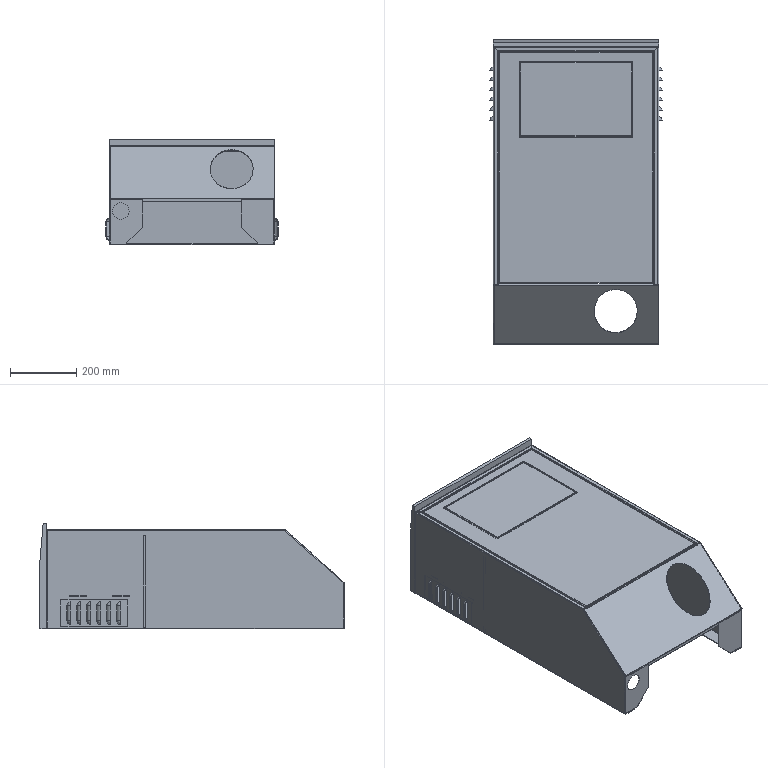Part | SolidWorks | features EdgeFlange 13, ICE 11, FlatPattern 7, SheetMetal 6, SMBaseFlange 5, LPattern 3, Cut 2, Chamfer 1, FormToolInstance 1, MirrorSolid 1, SolidToSheetMetal 1 | 12 solids | 574 faces | box 520 x 920 x 319.997 mm | volume 6254954 mm3 | plane 303 | cylinder 134 | spline 65 | sphere 48 | torus 24 | commonest cylinder face diameters 1.473 x38 5.473 x38 20 x24 4 x12 24 x12 2 x4